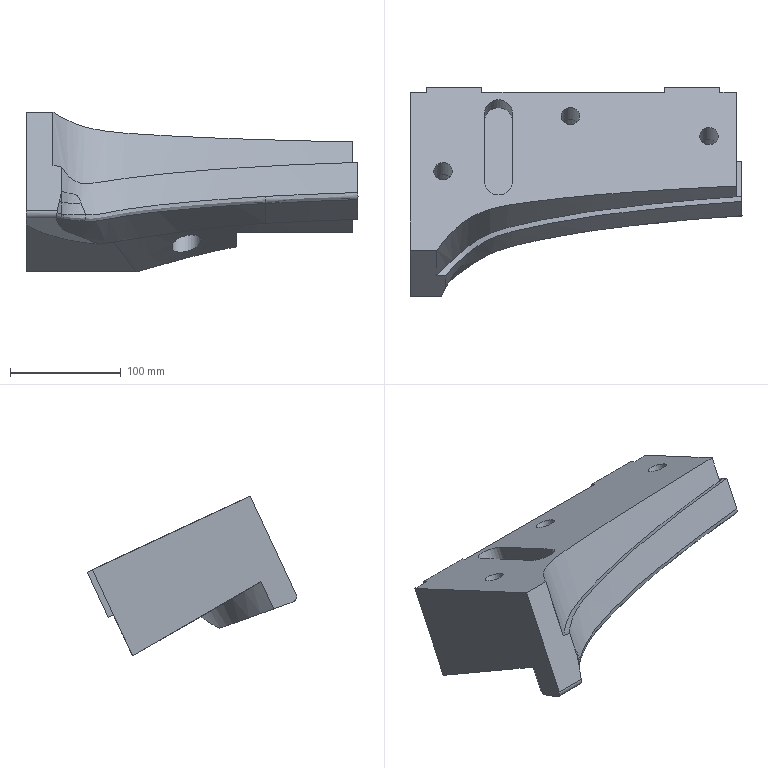Part | NX | features solid 2 | 1 solid | 52 faces | box 300 x 189.253 x 144.489 mm | volume 2328456 mm3 | plane 26 | spline 17 | cylinder 9 | commonest cylinder face diameters 17 x3 26 x3 25 x2 10 x1